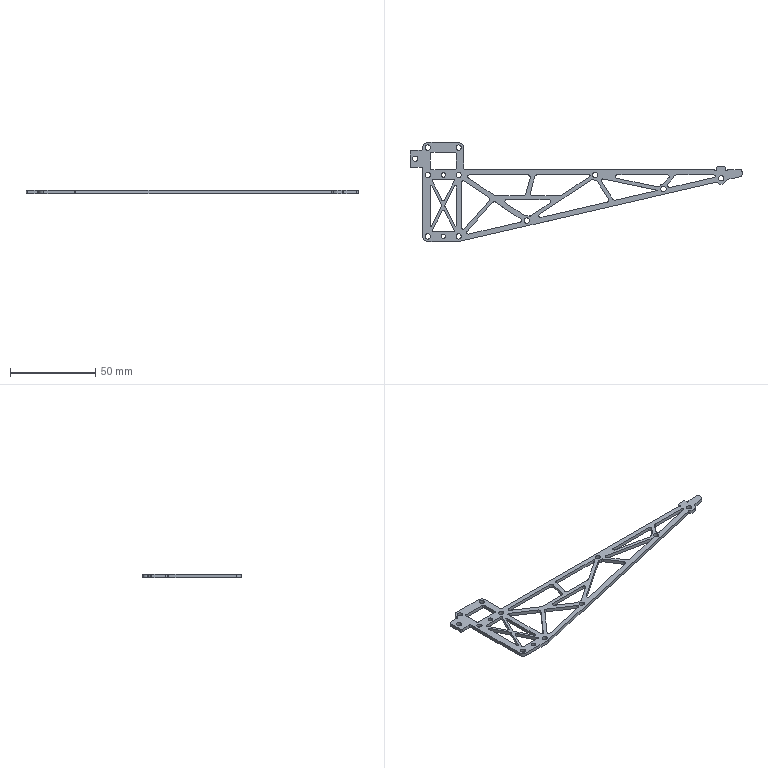Part | SolidWorks | features Fillet 5, ICE 2, Chamfer 1, Extrusion 1 | 1 solid | 173 faces | box 194.5 x 58 x 2 mm | volume 4743 mm3 | cylinder 108 | plane 65 | commonest cylinder face diameters 2 x48 3.1 x22 3 x13 1 x10 6 x8 2.6 x4